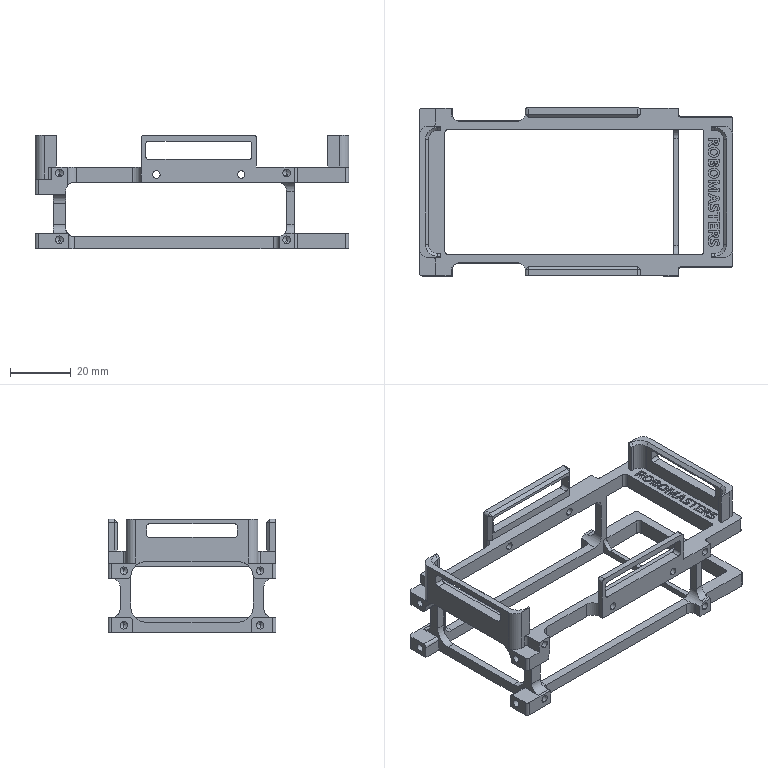Part | SolidWorks | features BaseBody 1 | 1 solid | 458 faces | box 103.5 x 55.4 x 37.5 mm | volume 17181 mm3 | plane 228 | cylinder 122 | spline 68 | cone 40 | commonest cylinder face diameters 2 x44 2.5 x40 6 x30 4 x4 10 x4